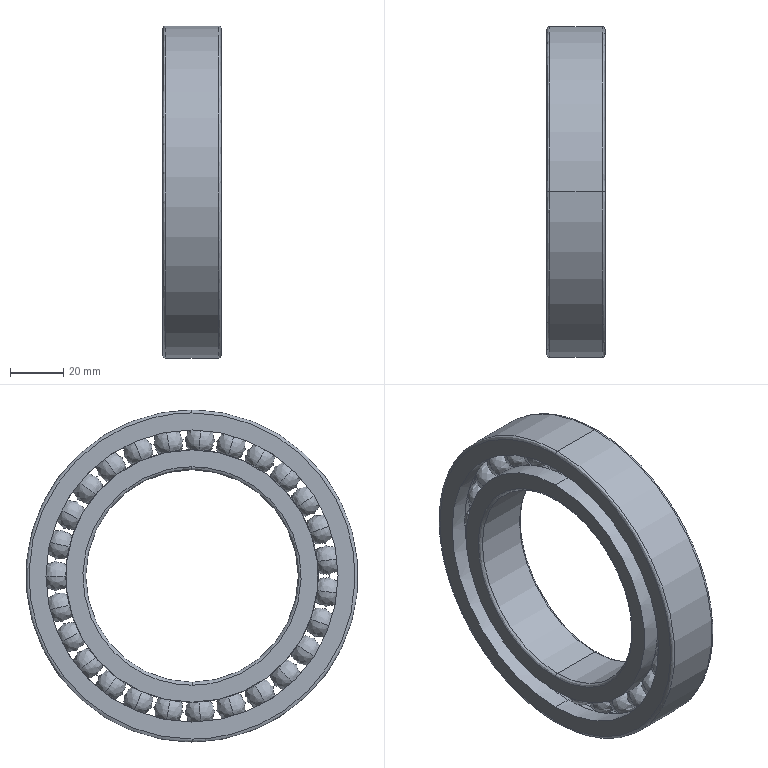Part | SolidWorks | features BaseBody 1 | 1 solid | 162 faces | box 22 x 125 x 125 mm | volume 119073 mm3 | spline 146 | cylinder 12 | plane 4 | commonest cylinder face diameters 95 x4 110 x4 80 x2 125 x2